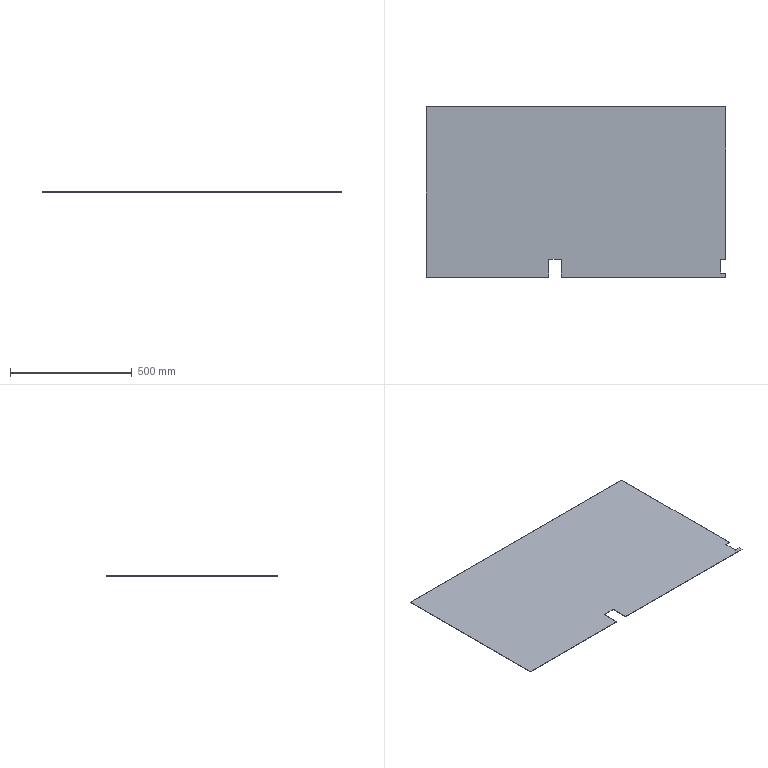Part | SolidWorks | 1 solid | 14 faces | box 1230 x 700 x 1.5 mm | volume 1284042 mm3 | plane 14
STEP:
#1=CARTESIAN_POINT('',(-615.,-350.,0.));
#2=VERTEX_POINT('',#1);
#3=CARTESIAN_POINT('',(-112.,-350.,0.));
#4=VERTEX_POINT('',#3);
#5=CARTESIAN_POINT('',(615.,-350.,0.));
#6=DIRECTION('',(1.,0.,0.));
#7=VECTOR('',#6,1000.);
#8=LINE('',#5,#7);
#9=EDGE_CURVE('',#2,#4,#8,.T.);
#10=ORIENTED_EDGE('',*,*,#9,.T.);
#11=CARTESIAN_POINT('',(-112.,-350.,1.5));
#12=VERTEX_POINT('',#11);
#13=CARTESIAN_POINT('',(-112.,-350.,-0.001));
#14=DIRECTION('',(0.,0.,-1.));
#15=VECTOR('',#14,1000.);
#16=LINE('',#13,#15);
#17=EDGE_CURVE('',#12,#4,#16,.T.);
#18=ORIENTED_EDGE('',*,*,#17,.F.);
#19=CARTESIAN_POINT('',(-615.,-350.,1.5));
#20=VERTEX_POINT('',#19);
#21=CARTESIAN_POINT('',(615.,-350.,1.5));
#22=DIRECTION('',(1.,0.,0.));
#23=VECTOR('',#22,1000.);
#24=LINE('',#21,#23);
#25=EDGE_CURVE('',#20,#12,#24,.T.);
#26=ORIENTED_EDGE('',*,*,#25,.F.);
#27=CARTESIAN_POINT('',(-615.,-350.,1.5));
#28=DIRECTION('',(0.,0.,-1.));
#29=VECTOR('',#28,1000.);
#30=LINE('',#27,#29);
#31=EDGE_CURVE('',#20,#2,#30,.T.);
#32=ORIENTED_EDGE('',*,*,#31,.T.);
#33=EDGE_LOOP('',(#10,#18,#26,#32));
#34=FACE_OUTER_BOUND('',#33,.T.);
#35=CARTESIAN_POINT('',(615.,-350.,1.5));
#36=DIRECTION('',(0.,1.,0.));
#37=DIRECTION('',(0.,0.,1.));
#38=AXIS2_PLACEMENT_3D('',#35,#36,#37);
#39=PLANE('',#38);
#40=ADVANCED_FACE('',(#34),#39,.F.);
#41=CARTESIAN_POINT('',(615.,-350.,0.));
#42=VERTEX_POINT('',#41);
#43=CARTESIAN_POINT('',(615.,-333.,0.));
#44=VERTEX_POINT('',#43);
#45=CARTESIAN_POINT('',(615.,-350.,0.));
#46=DIRECTION('',(0.,1.,0.));
#47=VECTOR('',#46,1000.);
#48=LINE('',#45,#47);
#49=EDGE_CURVE('',#42,#44,#48,.T.);
#50=ORIENTED_EDGE('',*,*,#49,.T.);
#51=CARTESIAN_POINT('',(615.,-333.,1.5));
#52=VERTEX_POINT('',#51);
#53=CARTESIAN_POINT('',(615.,-333.,-0.001));
#54=DIRECTION('',(0.,0.,-1.));
#55=VECTOR('',#54,1000.);
#56=LINE('',#53,#55);
#57=EDGE_CURVE('',#52,#44,#56,.T.);
#58=ORIENTED_EDGE('',*,*,#57,.F.);
#59=CARTESIAN_POINT('',(615.,-350.,1.5));
#60=VERTEX_POINT('',#59);
#61=CARTESIAN_POINT('',(615.,-350.,1.5));
#62=DIRECTION('',(0.,1.,0.));
#63=VECTOR('',#62,1000.);
#64=LINE('',#61,#63);
#65=EDGE_CURVE('',#60,#52,#64,.T.);
#66=ORIENTED_EDGE('',*,*,#65,.F.);
#67=CARTESIAN_POINT('',(615.,-350.,1.5));
#68=DIRECTION('',(0.,0.,-1.));
#69=VECTOR('',#68,1000.);
#70=LINE('',#67,#69);
#71=EDGE_CURVE('',#60,#42,#70,.T.);
#72=ORIENTED_EDGE('',*,*,#71,.T.);
#73=EDGE_LOOP('',(#50,#58,#66,#72));
#74=FACE_OUTER_BOUND('',#73,.T.);
#75=CARTESIAN_POINT('',(615.,-350.,1.5));
#76=DIRECTION('',(-1.,0.,0.));
#77=DIRECTION('',(0.,0.,1.));
#78=AXIS2_PLACEMENT_3D('',#75,#76,#77);
#79=PLANE('',#78);
#80=ADVANCED_FACE('',(#74),#79,.F.);
#81=CARTESIAN_POINT('',(615.,-277.,1.5));
#82=VERTEX_POINT('',#81);
#83=CARTESIAN_POINT('',(615.,350.,1.5));
#84=VERTEX_POINT('',#83);
#85=CARTESIAN_POINT('',(615.,-350.,1.5));
#86=DIRECTION('',(0.,1.,0.));
#87=VECTOR('',#86,1000.);
#88=LINE('',#85,#87);
#89=EDGE_CURVE('',#82,#84,#88,.T.);
#90=ORIENTED_EDGE('',*,*,#89,.F.);
#91=CARTESIAN_POINT('',(615.,-277.,0.));
#92=VERTEX_POINT('',#91);
#93=CARTESIAN_POINT('',(615.,-277.,-0.001));
#94=DIRECTION('',(0.,0.,1.));
#95=VECTOR('',#94,1000.);
#96=LINE('',#93,#95);
#97=EDGE_CURVE('',#92,#82,#96,.T.);
#98=ORIENTED_EDGE('',*,*,#97,.F.);
#99=CARTESIAN_POINT('',(615.,350.,0.));
#100=VERTEX_POINT('',#99);
#101=CARTESIAN_POINT('',(615.,-350.,0.));
#102=DIRECTION('',(0.,1.,0.));
#103=VECTOR('',#102,1000.);
#104=LINE('',#101,#103);
#105=EDGE_CURVE('',#92,#100,#104,.T.);
#106=ORIENTED_EDGE('',*,*,#105,.T.);
#107=CARTESIAN_POINT('',(615.,350.,1.5));
#108=DIRECTION('',(0.,0.,-1.));
#109=VECTOR('',#108,1000.);
#110=LINE('',#107,#109);
#111=EDGE_CURVE('',#84,#100,#110,.T.);
#112=ORIENTED_EDGE('',*,*,#111,.F.);
#113=EDGE_LOOP('',(#90,#98,#106,#112));
#114=FACE_OUTER_BOUND('',#113,.T.);
#115=CARTESIAN_POINT('',(615.,-350.,1.5));
#116=DIRECTION('',(-1.,0.,0.));
#117=DIRECTION('',(0.,0.,1.));
#118=AXIS2_PLACEMENT_3D('',#115,#116,#117);
#119=PLANE('',#118);
#120=ADVANCED_FACE('',(#114),#119,.F.);
#121=CARTESIAN_POINT('',(-615.,350.,0.));
#122=VERTEX_POINT('',#121);
#123=CARTESIAN_POINT('',(615.,350.,0.));
#124=DIRECTION('',(-1.,0.,0.));
#125=VECTOR('',#124,1000.);
#126=LINE('',#123,#125);
#127=EDGE_CURVE('',#100,#122,#126,.T.);
#128=ORIENTED_EDGE('',*,*,#127,.T.);
#129=CARTESIAN_POINT('',(-615.,350.,1.5));
#130=VERTEX_POINT('',#129);
#131=CARTESIAN_POINT('',(-615.,350.,1.5));
#132=DIRECTION('',(0.,0.,-1.));
#133=VECTOR('',#132,1000.);
#134=LINE('',#131,#133);
#135=EDGE_CURVE('',#130,#122,#134,.T.);
#136=ORIENTED_EDGE('',*,*,#135,.F.);
#137=CARTESIAN_POINT('',(615.,350.,1.5));
#138=DIRECTION('',(-1.,0.,0.));
#139=VECTOR('',#138,1000.);
#140=LINE('',#137,#139);
#141=EDGE_CURVE('',#84,#130,#140,.T.);
#142=ORIENTED_EDGE('',*,*,#141,.F.);
#143=ORIENTED_EDGE('',*,*,#111,.T.);
#144=EDGE_LOOP('',(#128,#136,#142,#143));
#145=FACE_OUTER_BOUND('',#144,.T.);
#146=CARTESIAN_POINT('',(615.,350.,1.5));
#147=DIRECTION('',(0.,-1.,0.));
#148=DIRECTION('',(0.,0.,-1.));
#149=AXIS2_PLACEMENT_3D('',#146,#147,#148);
#150=PLANE('',#149);
#151=ADVANCED_FACE('',(#145),#150,.F.);
#152=CARTESIAN_POINT('',(-615.,-350.,0.));
#153=DIRECTION('',(0.,-1.,0.));
#154=VECTOR('',#153,1000.);
#155=LINE('',#152,#154);
#156=EDGE_CURVE('',#122,#2,#155,.T.);
#157=ORIENTED_EDGE('',*,*,#156,.T.);
#158=ORIENTED_EDGE('',*,*,#31,.F.);
#159=CARTESIAN_POINT('',(-615.,-350.,1.5));
#160=DIRECTION('',(0.,-1.,0.));
#161=VECTOR('',#160,1000.);
#162=LINE('',#159,#161);
#163=EDGE_CURVE('',#130,#20,#162,.T.);
#164=ORIENTED_EDGE('',*,*,#163,.F.);
#165=ORIENTED_EDGE('',*,*,#135,.T.);
#166=EDGE_LOOP('',(#157,#158,#164,#165));
#167=FACE_OUTER_BOUND('',#166,.T.);
#168=CARTESIAN_POINT('',(-615.,-350.,1.5));
#169=DIRECTION('',(1.,0.,0.));
#170=DIRECTION('',(0.,0.,-1.));
#171=AXIS2_PLACEMENT_3D('',#168,#169,#170);
#172=PLANE('',#171);
#173=ADVANCED_FACE('',(#167),#172,.F.);
#174=CARTESIAN_POINT('',(-60.,-350.,1.5));
#175=VERTEX_POINT('',#174);
#176=CARTESIAN_POINT('',(615.,-350.,1.5));
#177=DIRECTION('',(1.,0.,0.));
#178=VECTOR('',#177,1000.);
#179=LINE('',#176,#178);
#180=EDGE_CURVE('',#175,#60,#179,.T.);
#181=ORIENTED_EDGE('',*,*,#180,.F.);
#182=CARTESIAN_POINT('',(-60.,-350.,0.));
#183=VERTEX_POINT('',#182);
#184=CARTESIAN_POINT('',(-60.,-350.,-0.001));
#185=DIRECTION('',(0.,0.,1.));
#186=VECTOR('',#185,1000.);
#187=LINE('',#184,#186);
#188=EDGE_CURVE('',#183,#175,#187,.T.);
#189=ORIENTED_EDGE('',*,*,#188,.F.);
#190=CARTESIAN_POINT('',(615.,-350.,0.));
#191=DIRECTION('',(1.,0.,0.));
#192=VECTOR('',#191,1000.);
#193=LINE('',#190,#192);
#194=EDGE_CURVE('',#183,#42,#193,.T.);
#195=ORIENTED_EDGE('',*,*,#194,.T.);
#196=ORIENTED_EDGE('',*,*,#71,.F.);
#197=EDGE_LOOP('',(#181,#189,#195,#196));
#198=FACE_OUTER_BOUND('',#197,.T.);
#199=CARTESIAN_POINT('',(615.,-350.,1.5));
#200=DIRECTION('',(0.,1.,0.));
#201=DIRECTION('',(0.,0.,1.));
#202=AXIS2_PLACEMENT_3D('',#199,#200,#201);
#203=PLANE('',#202);
#204=ADVANCED_FACE('',(#198),#203,.F.);
#205=CARTESIAN_POINT('',(-112.,-277.,1.5));
#206=VERTEX_POINT('',#205);
#207=CARTESIAN_POINT('',(-112.,-277.,1.5));
#208=DIRECTION('',(0.,-1.,0.));
#209=VECTOR('',#208,1000.);
#210=LINE('',#207,#209);
#211=EDGE_CURVE('',#206,#12,#210,.T.);
#212=ORIENTED_EDGE('',*,*,#211,.F.);
#213=CARTESIAN_POINT('',(-60.,-277.,1.5));
#214=VERTEX_POINT('',#213);
#215=CARTESIAN_POINT('',(-112.,-277.,1.5));
#216=DIRECTION('',(-1.,0.,0.));
#217=VECTOR('',#216,1000.);
#218=LINE('',#215,#217);
#219=EDGE_CURVE('',#214,#206,#218,.T.);
#220=ORIENTED_EDGE('',*,*,#219,.F.);
#221=CARTESIAN_POINT('',(-60.,-277.,1.5));
#222=DIRECTION('',(0.,1.,0.));
#223=VECTOR('',#222,1000.);
#224=LINE('',#221,#223);
#225=EDGE_CURVE('',#175,#214,#224,.T.);
#226=ORIENTED_EDGE('',*,*,#225,.F.);
#227=ORIENTED_EDGE('',*,*,#180,.T.);
#228=ORIENTED_EDGE('',*,*,#65,.T.);
#229=CARTESIAN_POINT('',(594.,-333.,1.5));
#230=VERTEX_POINT('',#229);
#231=CARTESIAN_POINT('',(644.,-333.,1.5));
#232=DIRECTION('',(1.,0.,0.));
#233=VECTOR('',#232,1000.);
#234=LINE('',#231,#233);
#235=EDGE_CURVE('',#230,#52,#234,.T.);
#236=ORIENTED_EDGE('',*,*,#235,.F.);
#237=CARTESIAN_POINT('',(594.,-277.,1.5));
#238=VERTEX_POINT('',#237);
#239=CARTESIAN_POINT('',(594.,-277.,1.5));
#240=DIRECTION('',(0.,-1.,0.));
#241=VECTOR('',#240,1000.);
#242=LINE('',#239,#241);
#243=EDGE_CURVE('',#238,#230,#242,.T.);
#244=ORIENTED_EDGE('',*,*,#243,.F.);
#245=CARTESIAN_POINT('',(644.,-277.,1.5));
#246=DIRECTION('',(-1.,0.,0.));
#247=VECTOR('',#246,1000.);
#248=LINE('',#245,#247);
#249=EDGE_CURVE('',#82,#238,#248,.T.);
#250=ORIENTED_EDGE('',*,*,#249,.F.);
#251=ORIENTED_EDGE('',*,*,#89,.T.);
#252=ORIENTED_EDGE('',*,*,#141,.T.);
#253=ORIENTED_EDGE('',*,*,#163,.T.);
#254=ORIENTED_EDGE('',*,*,#25,.T.);
#255=EDGE_LOOP('',(#212,#220,#226,#227,#228,#236,#244,#250,#251,#252,#253,#254));
#256=FACE_OUTER_BOUND('',#255,.T.);
#257=CARTESIAN_POINT('',(0.,0.,1.5));
#258=DIRECTION('',(0.,0.,1.));
#259=DIRECTION('',(1.,0.,0.));
#260=AXIS2_PLACEMENT_3D('',#257,#258,#259);
#261=PLANE('',#260);
#262=ADVANCED_FACE('',(#256),#261,.T.);
#263=CARTESIAN_POINT('',(-112.,-277.,0.));
#264=VERTEX_POINT('',#263);
#265=CARTESIAN_POINT('',(-60.,-277.,0.));
#266=VERTEX_POINT('',#265);
#267=CARTESIAN_POINT('',(-112.,-277.,0.));
#268=DIRECTION('',(1.,0.,0.));
#269=VECTOR('',#268,1000.);
#270=LINE('',#267,#269);
#271=EDGE_CURVE('',#264,#266,#270,.T.);
#272=ORIENTED_EDGE('',*,*,#271,.F.);
#273=CARTESIAN_POINT('',(-112.,-277.,0.));
#274=DIRECTION('',(0.,1.,0.));
#275=VECTOR('',#274,1000.);
#276=LINE('',#273,#275);
#277=EDGE_CURVE('',#4,#264,#276,.T.);
#278=ORIENTED_EDGE('',*,*,#277,.F.);
#279=ORIENTED_EDGE('',*,*,#9,.F.);
#280=ORIENTED_EDGE('',*,*,#156,.F.);
#281=ORIENTED_EDGE('',*,*,#127,.F.);
#282=ORIENTED_EDGE('',*,*,#105,.F.);
#283=CARTESIAN_POINT('',(594.,-277.,0.));
#284=VERTEX_POINT('',#283);
#285=CARTESIAN_POINT('',(644.,-277.,0.));
#286=DIRECTION('',(1.,0.,0.));
#287=VECTOR('',#286,1000.);
#288=LINE('',#285,#287);
#289=EDGE_CURVE('',#284,#92,#288,.T.);
#290=ORIENTED_EDGE('',*,*,#289,.F.);
#291=CARTESIAN_POINT('',(594.,-333.,0.));
#292=VERTEX_POINT('',#291);
#293=CARTESIAN_POINT('',(594.,-277.,0.));
#294=DIRECTION('',(0.,1.,0.));
#295=VECTOR('',#294,1000.);
#296=LINE('',#293,#295);
#297=EDGE_CURVE('',#292,#284,#296,.T.);
#298=ORIENTED_EDGE('',*,*,#297,.F.);
#299=CARTESIAN_POINT('',(644.,-333.,0.));
#300=DIRECTION('',(-1.,0.,0.));
#301=VECTOR('',#300,1000.);
#302=LINE('',#299,#301);
#303=EDGE_CURVE('',#44,#292,#302,.T.);
#304=ORIENTED_EDGE('',*,*,#303,.F.);
#305=ORIENTED_EDGE('',*,*,#49,.F.);
#306=ORIENTED_EDGE('',*,*,#194,.F.);
#307=CARTESIAN_POINT('',(-60.,-277.,0.));
#308=DIRECTION('',(0.,-1.,0.));
#309=VECTOR('',#308,1000.);
#310=LINE('',#307,#309);
#311=EDGE_CURVE('',#266,#183,#310,.T.);
#312=ORIENTED_EDGE('',*,*,#311,.F.);
#313=EDGE_LOOP('',(#272,#278,#279,#280,#281,#282,#290,#298,#304,#305,#306,#312));
#314=FACE_OUTER_BOUND('',#313,.T.);
#315=CARTESIAN_POINT('',(0.,0.,0.));
#316=DIRECTION('',(0.,0.,1.));
#317=DIRECTION('',(1.,0.,0.));
#318=AXIS2_PLACEMENT_3D('',#315,#316,#317);
#319=PLANE('',#318);
#320=ADVANCED_FACE('',(#314),#319,.F.);
#321=ORIENTED_EDGE('',*,*,#57,.T.);
#322=ORIENTED_EDGE('',*,*,#303,.T.);
#323=CARTESIAN_POINT('',(594.,-333.,-0.001));
#324=DIRECTION('',(0.,0.,1.));
#325=VECTOR('',#324,1000.);
#326=LINE('',#323,#325);
#327=EDGE_CURVE('',#292,#230,#326,.T.);
#328=ORIENTED_EDGE('',*,*,#327,.T.);
#329=ORIENTED_EDGE('',*,*,#235,.T.);
#330=EDGE_LOOP('',(#321,#322,#328,#329));
#331=FACE_OUTER_BOUND('',#330,.T.);
#332=CARTESIAN_POINT('',(644.,-333.,-0.001));
#333=DIRECTION('',(0.,-1.,0.));
#334=DIRECTION('',(0.,0.,-1.));
#335=AXIS2_PLACEMENT_3D('',#332,#333,#334);
#336=PLANE('',#335);
#337=ADVANCED_FACE('',(#331),#336,.F.);
#338=ORIENTED_EDGE('',*,*,#297,.T.);
#339=CARTESIAN_POINT('',(594.,-277.,-0.001));
#340=DIRECTION('',(0.,0.,1.));
#341=VECTOR('',#340,1000.);
#342=LINE('',#339,#341);
#343=EDGE_CURVE('',#284,#238,#342,.T.);
#344=ORIENTED_EDGE('',*,*,#343,.T.);
#345=ORIENTED_EDGE('',*,*,#243,.T.);
#346=ORIENTED_EDGE('',*,*,#327,.F.);
#347=EDGE_LOOP('',(#338,#344,#345,#346));
#348=FACE_OUTER_BOUND('',#347,.T.);
#349=CARTESIAN_POINT('',(594.,-277.,-0.001));
#350=DIRECTION('',(-1.,0.,0.));
#351=DIRECTION('',(0.,0.,1.));
#352=AXIS2_PLACEMENT_3D('',#349,#350,#351);
#353=PLANE('',#352);
#354=ADVANCED_FACE('',(#348),#353,.F.);
#355=ORIENTED_EDGE('',*,*,#97,.T.);
#356=ORIENTED_EDGE('',*,*,#249,.T.);
#357=ORIENTED_EDGE('',*,*,#343,.F.);
#358=ORIENTED_EDGE('',*,*,#289,.T.);
#359=EDGE_LOOP('',(#355,#356,#357,#358));
#360=FACE_OUTER_BOUND('',#359,.T.);
#361=CARTESIAN_POINT('',(644.,-277.,-0.001));
#362=DIRECTION('',(0.,1.,0.));
#363=DIRECTION('',(0.,0.,1.));
#364=AXIS2_PLACEMENT_3D('',#361,#362,#363);
#365=PLANE('',#364);
#366=ADVANCED_FACE('',(#360),#365,.F.);
#367=ORIENTED_EDGE('',*,*,#17,.T.);
#368=ORIENTED_EDGE('',*,*,#277,.T.);
#369=CARTESIAN_POINT('',(-112.,-277.,-0.001));
#370=DIRECTION('',(0.,0.,1.));
#371=VECTOR('',#370,1000.);
#372=LINE('',#369,#371);
#373=EDGE_CURVE('',#264,#206,#372,.T.);
#374=ORIENTED_EDGE('',*,*,#373,.T.);
#375=ORIENTED_EDGE('',*,*,#211,.T.);
#376=EDGE_LOOP('',(#367,#368,#374,#375));
#377=FACE_OUTER_BOUND('',#376,.T.);
#378=CARTESIAN_POINT('',(-112.,-277.,-0.001));
#379=DIRECTION('',(-1.,0.,0.));
#380=DIRECTION('',(0.,-1.,0.));
#381=AXIS2_PLACEMENT_3D('',#378,#379,#380);
#382=PLANE('',#381);
#383=ADVANCED_FACE('',(#377),#382,.F.);
#384=ORIENTED_EDGE('',*,*,#271,.T.);
#385=CARTESIAN_POINT('',(-60.,-277.,-0.001));
#386=DIRECTION('',(0.,0.,1.));
#387=VECTOR('',#386,1000.);
#388=LINE('',#385,#387);
#389=EDGE_CURVE('',#266,#214,#388,.T.);
#390=ORIENTED_EDGE('',*,*,#389,.T.);
#391=ORIENTED_EDGE('',*,*,#219,.T.);
#392=ORIENTED_EDGE('',*,*,#373,.F.);
#393=EDGE_LOOP('',(#384,#390,#391,#392));
#394=FACE_OUTER_BOUND('',#393,.T.);
#395=CARTESIAN_POINT('',(-112.,-277.,-0.001));
#396=DIRECTION('',(0.,1.,0.));
#397=DIRECTION('',(0.,0.,1.));
#398=AXIS2_PLACEMENT_3D('',#395,#396,#397);
#399=PLANE('',#398);
#400=ADVANCED_FACE('',(#394),#399,.F.);
#401=ORIENTED_EDGE('',*,*,#188,.T.);
#402=ORIENTED_EDGE('',*,*,#225,.T.);
#403=ORIENTED_EDGE('',*,*,#389,.F.);
#404=ORIENTED_EDGE('',*,*,#311,.T.);
#405=EDGE_LOOP('',(#401,#402,#403,#404));
#406=FACE_OUTER_BOUND('',#405,.T.);
#407=CARTESIAN_POINT('',(-60.,-277.,-0.001));
#408=DIRECTION('',(1.,0.,0.));
#409=DIRECTION('',(0.,1.,0.));
#410=AXIS2_PLACEMENT_3D('',#407,#408,#409);
#411=PLANE('',#410);
#412=ADVANCED_FACE('',(#406),#411,.F.);
#413=CLOSED_SHELL('',(#40,#80,#120,#151,#173,#204,#262,#320,#337,#354,#366,#383,#400,#412));
#414=MANIFOLD_SOLID_BREP('',#413);
#415=CARTESIAN_POINT('',(0.,0.,0.));
#416=DIRECTION('',(0.,0.,1.));
#417=DIRECTION('',(1.,0.,0.));
#418=AXIS2_PLACEMENT_3D('',#415,#416,#417);
#419=(LENGTH_UNIT()NAMED_UNIT(*)SI_UNIT(.MILLI.,.METRE.));
#420=UNCERTAINTY_MEASURE_WITH_UNIT(LENGTH_MEASURE(0.00001),#419,'','');
#421=(NAMED_UNIT(*)PLANE_ANGLE_UNIT()SI_UNIT($,.RADIAN.));
#422=(NAMED_UNIT(*)SI_UNIT($,.STERADIAN.)SOLID_ANGLE_UNIT());
#423=(GEOMETRIC_REPRESENTATION_CONTEXT(3)GLOBAL_UNCERTAINTY_ASSIGNED_CONTEXT((#420))GLOBAL_UNIT_ASSIGNED_CONTEXT((#419,#421,#422))REPRESENTATION_CONTEXT('',''));
#424=ADVANCED_BREP_SHAPE_REPRESENTATION('',(#414,#418),#423);